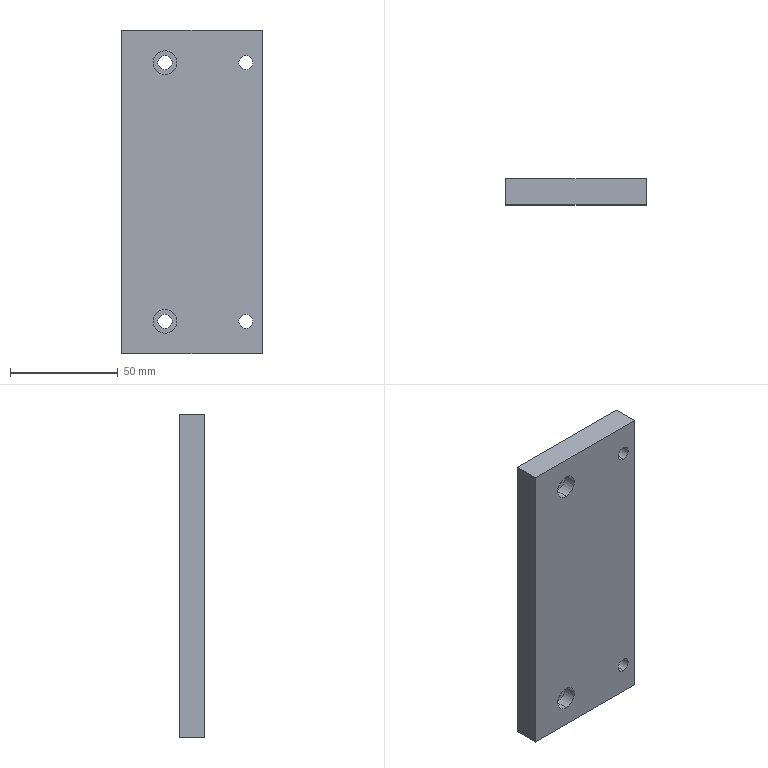Part | STEP file | 0245_208_Plate | 1 solid | 20 faces | box 65 x 12 x 150 mm | volume 114653 mm3 | cylinder 12 | plane 8 | commonest cylinder face diameters 6.5 x4 6.6 x4 11 x4